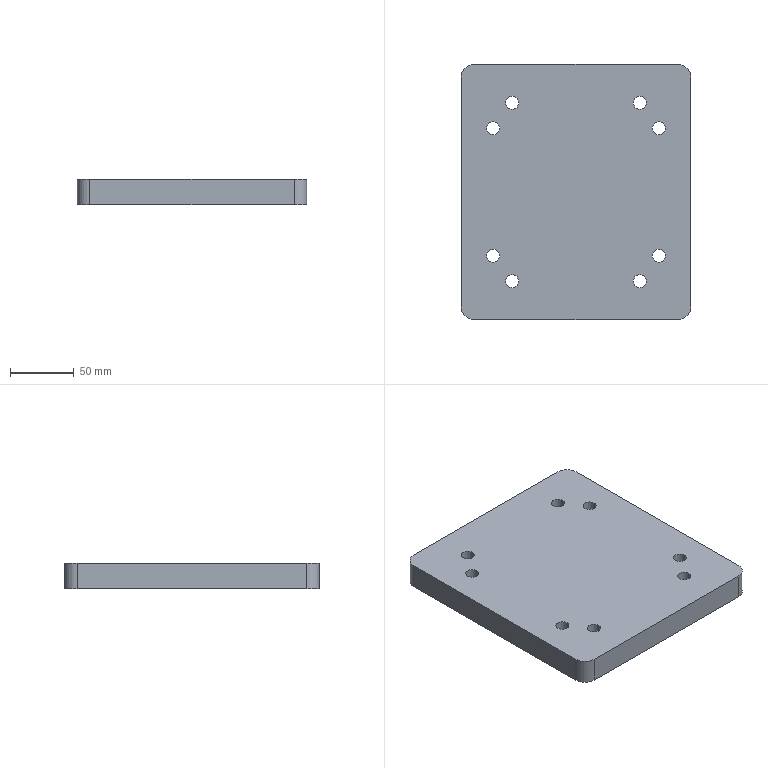Part | SolidWorks | features BaseBody 1 | 1 solid | 26 faces | box 180 x 200 x 20 mm | volume 705209 mm3 | cylinder 20 | plane 6 | commonest cylinder face diameters 10.2 x16 20 x4
STEP:
#1=CARTESIAN_POINT('',(-55.1,70.,-10.));
#2=VERTEX_POINT('',#1);
#3=CARTESIAN_POINT('',(-44.9,70.,-10.));
#4=VERTEX_POINT('',#3);
#5=CARTESIAN_POINT('',(-50.,70.,-10.));
#6=DIRECTION('',(0.,0.,1.));
#7=DIRECTION('',(1.,0.,0.));
#8=AXIS2_PLACEMENT_3D('',#5,#6,#7);
#9=CIRCLE('',#8,5.1);
#10=EDGE_CURVE('',#2,#4,#9,.T.);
#11=ORIENTED_EDGE('',*,*,#10,.F.);
#12=CARTESIAN_POINT('',(-55.1,70.,10.));
#13=VERTEX_POINT('',#12);
#14=CARTESIAN_POINT('',(-55.1,70.,10.));
#15=DIRECTION('',(0.,0.,1.));
#16=VECTOR('',#15,1000.);
#17=LINE('',#14,#16);
#18=EDGE_CURVE('',#2,#13,#17,.T.);
#19=ORIENTED_EDGE('',*,*,#18,.T.);
#20=CARTESIAN_POINT('',(-44.9,70.,10.));
#21=VERTEX_POINT('',#20);
#22=CARTESIAN_POINT('',(-50.,70.,10.));
#23=DIRECTION('',(0.,0.,1.));
#24=DIRECTION('',(1.,0.,0.));
#25=AXIS2_PLACEMENT_3D('',#22,#23,#24);
#26=CIRCLE('',#25,5.1);
#27=EDGE_CURVE('',#13,#21,#26,.T.);
#28=ORIENTED_EDGE('',*,*,#27,.T.);
#29=CARTESIAN_POINT('',(-44.9,70.,10.));
#30=DIRECTION('',(0.,0.,1.));
#31=VECTOR('',#30,1000.);
#32=LINE('',#29,#31);
#33=EDGE_CURVE('',#4,#21,#32,.T.);
#34=ORIENTED_EDGE('',*,*,#33,.F.);
#35=EDGE_LOOP('',(#11,#19,#28,#34));
#36=FACE_OUTER_BOUND('',#35,.T.);
#37=CARTESIAN_POINT('',(-50.,70.,10.));
#38=DIRECTION('',(0.,0.,1.));
#39=DIRECTION('',(1.,0.,0.));
#40=AXIS2_PLACEMENT_3D('',#37,#38,#39);
#41=CYLINDRICAL_SURFACE('',#40,5.1);
#42=ADVANCED_FACE('',(#36),#41,.F.);
#43=CARTESIAN_POINT('',(44.9,70.,-10.));
#44=VERTEX_POINT('',#43);
#45=CARTESIAN_POINT('',(55.1,70.,-10.));
#46=VERTEX_POINT('',#45);
#47=CARTESIAN_POINT('',(50.,70.,-10.));
#48=DIRECTION('',(0.,0.,1.));
#49=DIRECTION('',(1.,0.,0.));
#50=AXIS2_PLACEMENT_3D('',#47,#48,#49);
#51=CIRCLE('',#50,5.1);
#52=EDGE_CURVE('',#44,#46,#51,.T.);
#53=ORIENTED_EDGE('',*,*,#52,.F.);
#54=CARTESIAN_POINT('',(44.9,70.,10.));
#55=VERTEX_POINT('',#54);
#56=CARTESIAN_POINT('',(44.9,70.,10.));
#57=DIRECTION('',(0.,0.,1.));
#58=VECTOR('',#57,1000.);
#59=LINE('',#56,#58);
#60=EDGE_CURVE('',#44,#55,#59,.T.);
#61=ORIENTED_EDGE('',*,*,#60,.T.);
#62=CARTESIAN_POINT('',(55.1,70.,10.));
#63=VERTEX_POINT('',#62);
#64=CARTESIAN_POINT('',(50.,70.,10.));
#65=DIRECTION('',(0.,0.,1.));
#66=DIRECTION('',(1.,0.,0.));
#67=AXIS2_PLACEMENT_3D('',#64,#65,#66);
#68=CIRCLE('',#67,5.1);
#69=EDGE_CURVE('',#55,#63,#68,.T.);
#70=ORIENTED_EDGE('',*,*,#69,.T.);
#71=CARTESIAN_POINT('',(55.1,70.,10.));
#72=DIRECTION('',(0.,0.,1.));
#73=VECTOR('',#72,1000.);
#74=LINE('',#71,#73);
#75=EDGE_CURVE('',#46,#63,#74,.T.);
#76=ORIENTED_EDGE('',*,*,#75,.F.);
#77=EDGE_LOOP('',(#53,#61,#70,#76));
#78=FACE_OUTER_BOUND('',#77,.T.);
#79=CARTESIAN_POINT('',(50.,70.,10.));
#80=DIRECTION('',(0.,0.,1.));
#81=DIRECTION('',(1.,0.,0.));
#82=AXIS2_PLACEMENT_3D('',#79,#80,#81);
#83=CYLINDRICAL_SURFACE('',#82,5.1);
#84=ADVANCED_FACE('',(#78),#83,.F.);
#85=CARTESIAN_POINT('',(44.9,-70.,-10.));
#86=VERTEX_POINT('',#85);
#87=CARTESIAN_POINT('',(55.1,-70.,-10.));
#88=VERTEX_POINT('',#87);
#89=CARTESIAN_POINT('',(50.,-70.,-10.));
#90=DIRECTION('',(0.,0.,1.));
#91=DIRECTION('',(1.,0.,0.));
#92=AXIS2_PLACEMENT_3D('',#89,#90,#91);
#93=CIRCLE('',#92,5.1);
#94=EDGE_CURVE('',#86,#88,#93,.T.);
#95=ORIENTED_EDGE('',*,*,#94,.F.);
#96=CARTESIAN_POINT('',(44.9,-70.,10.));
#97=VERTEX_POINT('',#96);
#98=CARTESIAN_POINT('',(44.9,-70.,10.));
#99=DIRECTION('',(0.,0.,1.));
#100=VECTOR('',#99,1000.);
#101=LINE('',#98,#100);
#102=EDGE_CURVE('',#86,#97,#101,.T.);
#103=ORIENTED_EDGE('',*,*,#102,.T.);
#104=CARTESIAN_POINT('',(55.1,-70.,10.));
#105=VERTEX_POINT('',#104);
#106=CARTESIAN_POINT('',(50.,-70.,10.));
#107=DIRECTION('',(0.,0.,1.));
#108=DIRECTION('',(1.,0.,0.));
#109=AXIS2_PLACEMENT_3D('',#106,#107,#108);
#110=CIRCLE('',#109,5.1);
#111=EDGE_CURVE('',#97,#105,#110,.T.);
#112=ORIENTED_EDGE('',*,*,#111,.T.);
#113=CARTESIAN_POINT('',(55.1,-70.,10.));
#114=DIRECTION('',(0.,0.,1.));
#115=VECTOR('',#114,1000.);
#116=LINE('',#113,#115);
#117=EDGE_CURVE('',#88,#105,#116,.T.);
#118=ORIENTED_EDGE('',*,*,#117,.F.);
#119=EDGE_LOOP('',(#95,#103,#112,#118));
#120=FACE_OUTER_BOUND('',#119,.T.);
#121=CARTESIAN_POINT('',(50.,-70.,10.));
#122=DIRECTION('',(0.,0.,1.));
#123=DIRECTION('',(1.,0.,0.));
#124=AXIS2_PLACEMENT_3D('',#121,#122,#123);
#125=CYLINDRICAL_SURFACE('',#124,5.1);
#126=ADVANCED_FACE('',(#120),#125,.F.);
#127=CARTESIAN_POINT('',(-55.1,-70.,-10.));
#128=VERTEX_POINT('',#127);
#129=CARTESIAN_POINT('',(-44.9,-70.,-10.));
#130=VERTEX_POINT('',#129);
#131=CARTESIAN_POINT('',(-50.,-70.,-10.));
#132=DIRECTION('',(0.,0.,1.));
#133=DIRECTION('',(1.,0.,0.));
#134=AXIS2_PLACEMENT_3D('',#131,#132,#133);
#135=CIRCLE('',#134,5.1);
#136=EDGE_CURVE('',#128,#130,#135,.T.);
#137=ORIENTED_EDGE('',*,*,#136,.F.);
#138=CARTESIAN_POINT('',(-55.1,-70.,10.));
#139=VERTEX_POINT('',#138);
#140=CARTESIAN_POINT('',(-55.1,-70.,10.));
#141=DIRECTION('',(0.,0.,1.));
#142=VECTOR('',#141,1000.);
#143=LINE('',#140,#142);
#144=EDGE_CURVE('',#128,#139,#143,.T.);
#145=ORIENTED_EDGE('',*,*,#144,.T.);
#146=CARTESIAN_POINT('',(-44.9,-70.,10.));
#147=VERTEX_POINT('',#146);
#148=CARTESIAN_POINT('',(-50.,-70.,10.));
#149=DIRECTION('',(0.,0.,1.));
#150=DIRECTION('',(1.,0.,0.));
#151=AXIS2_PLACEMENT_3D('',#148,#149,#150);
#152=CIRCLE('',#151,5.1);
#153=EDGE_CURVE('',#139,#147,#152,.T.);
#154=ORIENTED_EDGE('',*,*,#153,.T.);
#155=CARTESIAN_POINT('',(-44.9,-70.,10.));
#156=DIRECTION('',(0.,0.,1.));
#157=VECTOR('',#156,1000.);
#158=LINE('',#155,#157);
#159=EDGE_CURVE('',#130,#147,#158,.T.);
#160=ORIENTED_EDGE('',*,*,#159,.F.);
#161=EDGE_LOOP('',(#137,#145,#154,#160));
#162=FACE_OUTER_BOUND('',#161,.T.);
#163=CARTESIAN_POINT('',(-50.,-70.,10.));
#164=DIRECTION('',(0.,0.,1.));
#165=DIRECTION('',(1.,0.,0.));
#166=AXIS2_PLACEMENT_3D('',#163,#164,#165);
#167=CYLINDRICAL_SURFACE('',#166,5.1);
#168=ADVANCED_FACE('',(#162),#167,.F.);
#169=CARTESIAN_POINT('',(-70.1,50.,-10.));
#170=VERTEX_POINT('',#169);
#171=CARTESIAN_POINT('',(-59.9,50.,-10.));
#172=VERTEX_POINT('',#171);
#173=CARTESIAN_POINT('',(-65.,50.,-10.));
#174=DIRECTION('',(0.,0.,1.));
#175=DIRECTION('',(1.,0.,0.));
#176=AXIS2_PLACEMENT_3D('',#173,#174,#175);
#177=CIRCLE('',#176,5.1);
#178=EDGE_CURVE('',#170,#172,#177,.T.);
#179=ORIENTED_EDGE('',*,*,#178,.F.);
#180=CARTESIAN_POINT('',(-70.1,50.,10.));
#181=VERTEX_POINT('',#180);
#182=CARTESIAN_POINT('',(-70.1,50.,10.));
#183=DIRECTION('',(0.,0.,1.));
#184=VECTOR('',#183,1000.);
#185=LINE('',#182,#184);
#186=EDGE_CURVE('',#170,#181,#185,.T.);
#187=ORIENTED_EDGE('',*,*,#186,.T.);
#188=CARTESIAN_POINT('',(-59.9,50.,10.));
#189=VERTEX_POINT('',#188);
#190=CARTESIAN_POINT('',(-65.,50.,10.));
#191=DIRECTION('',(0.,0.,1.));
#192=DIRECTION('',(1.,0.,0.));
#193=AXIS2_PLACEMENT_3D('',#190,#191,#192);
#194=CIRCLE('',#193,5.1);
#195=EDGE_CURVE('',#181,#189,#194,.T.);
#196=ORIENTED_EDGE('',*,*,#195,.T.);
#197=CARTESIAN_POINT('',(-59.9,50.,10.));
#198=DIRECTION('',(0.,0.,1.));
#199=VECTOR('',#198,1000.);
#200=LINE('',#197,#199);
#201=EDGE_CURVE('',#172,#189,#200,.T.);
#202=ORIENTED_EDGE('',*,*,#201,.F.);
#203=EDGE_LOOP('',(#179,#187,#196,#202));
#204=FACE_OUTER_BOUND('',#203,.T.);
#205=CARTESIAN_POINT('',(-65.,50.,10.));
#206=DIRECTION('',(0.,0.,1.));
#207=DIRECTION('',(1.,0.,0.));
#208=AXIS2_PLACEMENT_3D('',#205,#206,#207);
#209=CYLINDRICAL_SURFACE('',#208,5.1);
#210=ADVANCED_FACE('',(#204),#209,.F.);
#211=CARTESIAN_POINT('',(59.9,50.,-10.));
#212=VERTEX_POINT('',#211);
#213=CARTESIAN_POINT('',(70.1,50.,-10.));
#214=VERTEX_POINT('',#213);
#215=CARTESIAN_POINT('',(65.,50.,-10.));
#216=DIRECTION('',(0.,0.,1.));
#217=DIRECTION('',(1.,0.,0.));
#218=AXIS2_PLACEMENT_3D('',#215,#216,#217);
#219=CIRCLE('',#218,5.1);
#220=EDGE_CURVE('',#212,#214,#219,.T.);
#221=ORIENTED_EDGE('',*,*,#220,.F.);
#222=CARTESIAN_POINT('',(59.9,50.,10.));
#223=VERTEX_POINT('',#222);
#224=CARTESIAN_POINT('',(59.9,50.,10.));
#225=DIRECTION('',(0.,0.,1.));
#226=VECTOR('',#225,1000.);
#227=LINE('',#224,#226);
#228=EDGE_CURVE('',#212,#223,#227,.T.);
#229=ORIENTED_EDGE('',*,*,#228,.T.);
#230=CARTESIAN_POINT('',(70.1,50.,10.));
#231=VERTEX_POINT('',#230);
#232=CARTESIAN_POINT('',(65.,50.,10.));
#233=DIRECTION('',(0.,0.,1.));
#234=DIRECTION('',(1.,0.,0.));
#235=AXIS2_PLACEMENT_3D('',#232,#233,#234);
#236=CIRCLE('',#235,5.1);
#237=EDGE_CURVE('',#223,#231,#236,.T.);
#238=ORIENTED_EDGE('',*,*,#237,.T.);
#239=CARTESIAN_POINT('',(70.1,50.,10.));
#240=DIRECTION('',(0.,0.,1.));
#241=VECTOR('',#240,1000.);
#242=LINE('',#239,#241);
#243=EDGE_CURVE('',#214,#231,#242,.T.);
#244=ORIENTED_EDGE('',*,*,#243,.F.);
#245=EDGE_LOOP('',(#221,#229,#238,#244));
#246=FACE_OUTER_BOUND('',#245,.T.);
#247=CARTESIAN_POINT('',(65.,50.,10.));
#248=DIRECTION('',(0.,0.,1.));
#249=DIRECTION('',(1.,0.,0.));
#250=AXIS2_PLACEMENT_3D('',#247,#248,#249);
#251=CYLINDRICAL_SURFACE('',#250,5.1);
#252=ADVANCED_FACE('',(#246),#251,.F.);
#253=CARTESIAN_POINT('',(59.9,-50.,-10.));
#254=VERTEX_POINT('',#253);
#255=CARTESIAN_POINT('',(70.1,-50.,-10.));
#256=VERTEX_POINT('',#255);
#257=CARTESIAN_POINT('',(65.,-50.,-10.));
#258=DIRECTION('',(0.,0.,1.));
#259=DIRECTION('',(1.,0.,0.));
#260=AXIS2_PLACEMENT_3D('',#257,#258,#259);
#261=CIRCLE('',#260,5.1);
#262=EDGE_CURVE('',#254,#256,#261,.T.);
#263=ORIENTED_EDGE('',*,*,#262,.F.);
#264=CARTESIAN_POINT('',(59.9,-50.,10.));
#265=VERTEX_POINT('',#264);
#266=CARTESIAN_POINT('',(59.9,-50.,10.));
#267=DIRECTION('',(0.,0.,1.));
#268=VECTOR('',#267,1000.);
#269=LINE('',#266,#268);
#270=EDGE_CURVE('',#254,#265,#269,.T.);
#271=ORIENTED_EDGE('',*,*,#270,.T.);
#272=CARTESIAN_POINT('',(70.1,-50.,10.));
#273=VERTEX_POINT('',#272);
#274=CARTESIAN_POINT('',(65.,-50.,10.));
#275=DIRECTION('',(0.,0.,1.));
#276=DIRECTION('',(1.,0.,0.));
#277=AXIS2_PLACEMENT_3D('',#274,#275,#276);
#278=CIRCLE('',#277,5.1);
#279=EDGE_CURVE('',#265,#273,#278,.T.);
#280=ORIENTED_EDGE('',*,*,#279,.T.);
#281=CARTESIAN_POINT('',(70.1,-50.,10.));
#282=DIRECTION('',(0.,0.,1.));
#283=VECTOR('',#282,1000.);
#284=LINE('',#281,#283);
#285=EDGE_CURVE('',#256,#273,#284,.T.);
#286=ORIENTED_EDGE('',*,*,#285,.F.);
#287=EDGE_LOOP('',(#263,#271,#280,#286));
#288=FACE_OUTER_BOUND('',#287,.T.);
#289=CARTESIAN_POINT('',(65.,-50.,10.));
#290=DIRECTION('',(0.,0.,1.));
#291=DIRECTION('',(1.,0.,0.));
#292=AXIS2_PLACEMENT_3D('',#289,#290,#291);
#293=CYLINDRICAL_SURFACE('',#292,5.1);
#294=ADVANCED_FACE('',(#288),#293,.F.);
#295=CARTESIAN_POINT('',(-70.1,-50.,-10.));
#296=VERTEX_POINT('',#295);
#297=CARTESIAN_POINT('',(-59.9,-50.,-10.));
#298=VERTEX_POINT('',#297);
#299=CARTESIAN_POINT('',(-65.,-50.,-10.));
#300=DIRECTION('',(0.,0.,1.));
#301=DIRECTION('',(1.,0.,0.));
#302=AXIS2_PLACEMENT_3D('',#299,#300,#301);
#303=CIRCLE('',#302,5.1);
#304=EDGE_CURVE('',#296,#298,#303,.T.);
#305=ORIENTED_EDGE('',*,*,#304,.F.);
#306=CARTESIAN_POINT('',(-70.1,-50.,10.));
#307=VERTEX_POINT('',#306);
#308=CARTESIAN_POINT('',(-70.1,-50.,10.));
#309=DIRECTION('',(0.,0.,1.));
#310=VECTOR('',#309,1000.);
#311=LINE('',#308,#310);
#312=EDGE_CURVE('',#296,#307,#311,.T.);
#313=ORIENTED_EDGE('',*,*,#312,.T.);
#314=CARTESIAN_POINT('',(-59.9,-50.,10.));
#315=VERTEX_POINT('',#314);
#316=CARTESIAN_POINT('',(-65.,-50.,10.));
#317=DIRECTION('',(0.,0.,1.));
#318=DIRECTION('',(1.,0.,0.));
#319=AXIS2_PLACEMENT_3D('',#316,#317,#318);
#320=CIRCLE('',#319,5.1);
#321=EDGE_CURVE('',#307,#315,#320,.T.);
#322=ORIENTED_EDGE('',*,*,#321,.T.);
#323=CARTESIAN_POINT('',(-59.9,-50.,10.));
#324=DIRECTION('',(0.,0.,1.));
#325=VECTOR('',#324,1000.);
#326=LINE('',#323,#325);
#327=EDGE_CURVE('',#298,#315,#326,.T.);
#328=ORIENTED_EDGE('',*,*,#327,.F.);
#329=EDGE_LOOP('',(#305,#313,#322,#328));
#330=FACE_OUTER_BOUND('',#329,.T.);
#331=CARTESIAN_POINT('',(-65.,-50.,10.));
#332=DIRECTION('',(0.,0.,1.));
#333=DIRECTION('',(1.,0.,0.));
#334=AXIS2_PLACEMENT_3D('',#331,#332,#333);
#335=CYLINDRICAL_SURFACE('',#334,5.1);
#336=ADVANCED_FACE('',(#330),#335,.F.);
#337=CARTESIAN_POINT('',(90.,90.,-10.));
#338=VERTEX_POINT('',#337);
#339=CARTESIAN_POINT('',(80.,100.,-10.));
#340=VERTEX_POINT('',#339);
#341=CARTESIAN_POINT('',(80.,90.,-10.));
#342=DIRECTION('',(0.,0.,1.));
#343=DIRECTION('',(-1.,0.,0.));
#344=AXIS2_PLACEMENT_3D('',#341,#342,#343);
#345=CIRCLE('',#344,10.);
#346=EDGE_CURVE('',#338,#340,#345,.T.);
#347=ORIENTED_EDGE('',*,*,#346,.T.);
#348=CARTESIAN_POINT('',(80.,100.,10.));
#349=VERTEX_POINT('',#348);
#350=CARTESIAN_POINT('',(80.,100.,10.));
#351=DIRECTION('',(0.,0.,-1.));
#352=VECTOR('',#351,1000.);
#353=LINE('',#350,#352);
#354=EDGE_CURVE('',#349,#340,#353,.T.);
#355=ORIENTED_EDGE('',*,*,#354,.F.);
#356=CARTESIAN_POINT('',(90.,90.,10.));
#357=VERTEX_POINT('',#356);
#358=CARTESIAN_POINT('',(80.,90.,10.));
#359=DIRECTION('',(0.,0.,1.));
#360=DIRECTION('',(-1.,0.,0.));
#361=AXIS2_PLACEMENT_3D('',#358,#359,#360);
#362=CIRCLE('',#361,10.);
#363=EDGE_CURVE('',#357,#349,#362,.T.);
#364=ORIENTED_EDGE('',*,*,#363,.F.);
#365=CARTESIAN_POINT('',(90.,90.,10.));
#366=DIRECTION('',(0.,0.,-1.));
#367=VECTOR('',#366,1000.);
#368=LINE('',#365,#367);
#369=EDGE_CURVE('',#357,#338,#368,.T.);
#370=ORIENTED_EDGE('',*,*,#369,.T.);
#371=EDGE_LOOP('',(#347,#355,#364,#370));
#372=FACE_OUTER_BOUND('',#371,.T.);
#373=CARTESIAN_POINT('',(80.,90.,10.));
#374=DIRECTION('',(0.,0.,-1.));
#375=DIRECTION('',(-1.,0.,0.));
#376=AXIS2_PLACEMENT_3D('',#373,#374,#375);
#377=CYLINDRICAL_SURFACE('',#376,10.);
#378=ADVANCED_FACE('',(#372),#377,.T.);
#379=CARTESIAN_POINT('',(-80.,100.,-10.));
#380=VERTEX_POINT('',#379);
#381=CARTESIAN_POINT('',(-80.,100.,-10.));
#382=DIRECTION('',(-1.,0.,0.));
#383=VECTOR('',#382,1000.);
#384=LINE('',#381,#383);
#385=EDGE_CURVE('',#340,#380,#384,.T.);
#386=ORIENTED_EDGE('',*,*,#385,.T.);
#387=CARTESIAN_POINT('',(-80.,100.,10.));
#388=VERTEX_POINT('',#387);
#389=CARTESIAN_POINT('',(-80.,100.,10.));
#390=DIRECTION('',(0.,0.,-1.));
#391=VECTOR('',#390,1000.);
#392=LINE('',#389,#391);
#393=EDGE_CURVE('',#388,#380,#392,.T.);
#394=ORIENTED_EDGE('',*,*,#393,.F.);
#395=CARTESIAN_POINT('',(-80.,100.,10.));
#396=DIRECTION('',(-1.,0.,0.));
#397=VECTOR('',#396,1000.);
#398=LINE('',#395,#397);
#399=EDGE_CURVE('',#349,#388,#398,.T.);
#400=ORIENTED_EDGE('',*,*,#399,.F.);
#401=ORIENTED_EDGE('',*,*,#354,.T.);
#402=EDGE_LOOP('',(#386,#394,#400,#401));
#403=FACE_OUTER_BOUND('',#402,.T.);
#404=CARTESIAN_POINT('',(-80.,100.,10.));
#405=DIRECTION('',(0.,-1.,0.));
#406=DIRECTION('',(0.,0.,-1.));
#407=AXIS2_PLACEMENT_3D('',#404,#405,#406);
#408=PLANE('',#407);
#409=ADVANCED_FACE('',(#403),#408,.F.);
#410=CARTESIAN_POINT('',(-90.,90.,-10.));
#411=VERTEX_POINT('',#410);
#412=CARTESIAN_POINT('',(-80.,90.,-10.));
#413=DIRECTION('',(0.,0.,1.));
#414=DIRECTION('',(1.,0.,0.));
#415=AXIS2_PLACEMENT_3D('',#412,#413,#414);
#416=CIRCLE('',#415,10.);
#417=EDGE_CURVE('',#380,#411,#416,.T.);
#418=ORIENTED_EDGE('',*,*,#417,.T.);
#419=CARTESIAN_POINT('',(-90.,90.,10.));
#420=VERTEX_POINT('',#419);
#421=CARTESIAN_POINT('',(-90.,90.,10.));
#422=DIRECTION('',(0.,0.,-1.));
#423=VECTOR('',#422,1000.);
#424=LINE('',#421,#423);
#425=EDGE_CURVE('',#420,#411,#424,.T.);
#426=ORIENTED_EDGE('',*,*,#425,.F.);
#427=CARTESIAN_POINT('',(-80.,90.,10.));
#428=DIRECTION('',(0.,0.,1.));
#429=DIRECTION('',(1.,0.,0.));
#430=AXIS2_PLACEMENT_3D('',#427,#428,#429);
#431=CIRCLE('',#430,10.);
#432=EDGE_CURVE('',#388,#420,#431,.T.);
#433=ORIENTED_EDGE('',*,*,#432,.F.);
#434=ORIENTED_EDGE('',*,*,#393,.T.);
#435=EDGE_LOOP('',(#418,#426,#433,#434));
#436=FACE_OUTER_BOUND('',#435,.T.);
#437=CARTESIAN_POINT('',(-80.,90.,10.));
#438=DIRECTION('',(0.,0.,-1.));
#439=DIRECTION('',(-1.,0.,0.));
#440=AXIS2_PLACEMENT_3D('',#437,#438,#439);
#441=CYLINDRICAL_SURFACE('',#440,10.);
#442=ADVANCED_FACE('',(#436),#441,.T.);
#443=CARTESIAN_POINT('',(-90.,-90.,-10.));
#444=VERTEX_POINT('',#443);
#445=CARTESIAN_POINT('',(-90.,90.,-10.));
#446=DIRECTION('',(0.,-1.,0.));
#447=VECTOR('',#446,1000.);
#448=LINE('',#445,#447);
#449=EDGE_CURVE('',#411,#444,#448,.T.);
#450=ORIENTED_EDGE('',*,*,#449,.T.);
#451=CARTESIAN_POINT('',(-90.,-90.,10.));
#452=VERTEX_POINT('',#451);
#453=CARTESIAN_POINT('',(-90.,-90.,10.));
#454=DIRECTION('',(0.,0.,-1.));
#455=VECTOR('',#454,1000.);
#456=LINE('',#453,#455);
#457=EDGE_CURVE('',#452,#444,#456,.T.);
#458=ORIENTED_EDGE('',*,*,#457,.F.);
#459=CARTESIAN_POINT('',(-90.,90.,10.));
#460=DIRECTION('',(0.,-1.,0.));
#461=VECTOR('',#460,1000.);
#462=LINE('',#459,#461);
#463=EDGE_CURVE('',#420,#452,#462,.T.);
#464=ORIENTED_EDGE('',*,*,#463,.F.);
#465=ORIENTED_EDGE('',*,*,#425,.T.);
#466=EDGE_LOOP('',(#450,#458,#464,#465));
#467=FACE_OUTER_BOUND('',#466,.T.);
#468=CARTESIAN_POINT('',(-90.,90.,10.));
#469=DIRECTION('',(1.,0.,0.));
#470=DIRECTION('',(0.,1.,0.));
#471=AXIS2_PLACEMENT_3D('',#468,#469,#470);
#472=PLANE('',#471);
#473=ADVANCED_FACE('',(#467),#472,.F.);
#474=CARTESIAN_POINT('',(-80.,-100.,-10.));
#475=VERTEX_POINT('',#474);
#476=CARTESIAN_POINT('',(-80.,-90.,-10.));
#477=DIRECTION('',(0.,0.,1.));
#478=DIRECTION('',(1.,0.,0.));
#479=AXIS2_PLACEMENT_3D('',#476,#477,#478);
#480=CIRCLE('',#479,10.);
#481=EDGE_CURVE('',#444,#475,#480,.T.);
#482=ORIENTED_EDGE('',*,*,#481,.T.);
#483=CARTESIAN_POINT('',(-80.,-100.,10.));
#484=VERTEX_POINT('',#483);
#485=CARTESIAN_POINT('',(-80.,-100.,10.));
#486=DIRECTION('',(0.,0.,-1.));
#487=VECTOR('',#486,1000.);
#488=LINE('',#485,#487);
#489=EDGE_CURVE('',#484,#475,#488,.T.);
#490=ORIENTED_EDGE('',*,*,#489,.F.);
#491=CARTESIAN_POINT('',(-80.,-90.,10.));
#492=DIRECTION('',(0.,0.,1.));
#493=DIRECTION('',(1.,0.,0.));
#494=AXIS2_PLACEMENT_3D('',#491,#492,#493);
#495=CIRCLE('',#494,10.);
#496=EDGE_CURVE('',#452,#484,#495,.T.);
#497=ORIENTED_EDGE('',*,*,#496,.F.);
#498=ORIENTED_EDGE('',*,*,#457,.T.);
#499=EDGE_LOOP('',(#482,#490,#497,#498));
#500=FACE_OUTER_BOUND('',#499,.T.);
#501=CARTESIAN_POINT('',(-80.,-90.,10.));
#502=DIRECTION('',(0.,0.,-1.));
#503=DIRECTION('',(-1.,0.,0.));
#504=AXIS2_PLACEMENT_3D('',#501,#502,#503);
#505=CYLINDRICAL_SURFACE('',#504,10.);
#506=ADVANCED_FACE('',(#500),#505,.T.);
#507=CARTESIAN_POINT('',(80.,-100.,-10.));
#508=VERTEX_POINT('',#507);
#509=CARTESIAN_POINT('',(-80.,-100.,-10.));
#510=DIRECTION('',(1.,0.,0.));
#511=VECTOR('',#510,1000.);
#512=LINE('',#509,#511);
#513=EDGE_CURVE('',#475,#508,#512,.T.);
#514=ORIENTED_EDGE('',*,*,#513,.T.);
#515=CARTESIAN_POINT('',(80.,-100.,10.));
#516=VERTEX_POINT('',#515);
#517=CARTESIAN_POINT('',(80.,-100.,10.));
#518=DIRECTION('',(0.,0.,-1.));
#519=VECTOR('',#518,1000.);
#520=LINE('',#517,#519);
#521=EDGE_CURVE('',#516,#508,#520,.T.);
#522=ORIENTED_EDGE('',*,*,#521,.F.);
#523=CARTESIAN_POINT('',(-80.,-100.,10.));
#524=DIRECTION('',(1.,0.,0.));
#525=VECTOR('',#524,1000.);
#526=LINE('',#523,#525);
#527=EDGE_CURVE('',#484,#516,#526,.T.);
#528=ORIENTED_EDGE('',*,*,#527,.F.);
#529=ORIENTED_EDGE('',*,*,#489,.T.);
#530=EDGE_LOOP('',(#514,#522,#528,#529));
#531=FACE_OUTER_BOUND('',#530,.T.);
#532=CARTESIAN_POINT('',(-80.,-100.,10.));
#533=DIRECTION('',(0.,1.,0.));
#534=DIRECTION('',(0.,0.,1.));
#535=AXIS2_PLACEMENT_3D('',#532,#533,#534);
#536=PLANE('',#535);
#537=ADVANCED_FACE('',(#531),#536,.F.);
#538=CARTESIAN_POINT('',(90.,-90.,-10.));
#539=VERTEX_POINT('',#538);
#540=CARTESIAN_POINT('',(80.,-90.,-10.));
#541=DIRECTION('',(0.,0.,1.));
#542=DIRECTION('',(1.,0.,0.));
#543=AXIS2_PLACEMENT_3D('',#540,#541,#542);
#544=CIRCLE('',#543,10.);
#545=EDGE_CURVE('',#508,#539,#544,.T.);
#546=ORIENTED_EDGE('',*,*,#545,.T.);
#547=CARTESIAN_POINT('',(90.,-90.,10.));
#548=VERTEX_POINT('',#547);
#549=CARTESIAN_POINT('',(90.,-90.,10.));
#550=DIRECTION('',(0.,0.,-1.));
#551=VECTOR('',#550,1000.);
#552=LINE('',#549,#551);
#553=EDGE_CURVE('',#548,#539,#552,.T.);
#554=ORIENTED_EDGE('',*,*,#553,.F.);
#555=CARTESIAN_POINT('',(80.,-90.,10.));
#556=DIRECTION('',(0.,0.,1.));
#557=DIRECTION('',(1.,0.,0.));
#558=AXIS2_PLACEMENT_3D('',#555,#556,#557);
#559=CIRCLE('',#558,10.);
#560=EDGE_CURVE('',#516,#548,#559,.T.);
#561=ORIENTED_EDGE('',*,*,#560,.F.);
#562=ORIENTED_EDGE('',*,*,#521,.T.);
#563=EDGE_LOOP('',(#546,#554,#561,#562));
#564=FACE_OUTER_BOUND('',#563,.T.);
#565=CARTESIAN_POINT('',(80.,-90.,10.));
#566=DIRECTION('',(0.,0.,-1.));
#567=DIRECTION('',(-1.,0.,0.));
#568=AXIS2_PLACEMENT_3D('',#565,#566,#567);
#569=CYLINDRICAL_SURFACE('',#568,10.);
#570=ADVANCED_FACE('',(#564),#569,.T.);
#571=CARTESIAN_POINT('',(90.,90.,-10.));
#572=DIRECTION('',(0.,1.,0.));
#573=VECTOR('',#572,1000.);
#574=LINE('',#571,#573);
#575=EDGE_CURVE('',#539,#338,#574,.T.);
#576=ORIENTED_EDGE('',*,*,#575,.T.);
#577=ORIENTED_EDGE('',*,*,#369,.F.);
#578=CARTESIAN_POINT('',(90.,90.,10.));
#579=DIRECTION('',(0.,1.,0.));
#580=VECTOR('',#579,1000.);
#581=LINE('',#578,#580);
#582=EDGE_CURVE('',#548,#357,#581,.T.);
#583=ORIENTED_EDGE('',*,*,#582,.F.);
#584=ORIENTED_EDGE('',*,*,#553,.T.);
#585=EDGE_LOOP('',(#576,#577,#583,#584));
#586=FACE_OUTER_BOUND('',#585,.T.);
#587=CARTESIAN_POINT('',(90.,90.,10.));
#588=DIRECTION('',(-1.,0.,0.));
#589=DIRECTION('',(0.,-1.,0.));
#590=AXIS2_PLACEMENT_3D('',#587,#588,#589);
#591=PLANE('',#590);
#592=ADVANCED_FACE('',(#586),#591,.F.);
#593=CARTESIAN_POINT('',(-50.,70.,10.));
#594=DIRECTION('',(0.,0.,1.));
#595=DIRECTION('',(1.,0.,0.));
#596=AXIS2_PLACEMENT_3D('',#593,#594,#595);
#597=CIRCLE('',#596,5.1);
#598=EDGE_CURVE('',#21,#13,#597,.T.);
#599=ORIENTED_EDGE('',*,*,#598,.F.);
#600=ORIENTED_EDGE('',*,*,#27,.F.);
#601=EDGE_LOOP('',(#599,#600));
#602=FACE_BOUND('',#601,.T.);
#603=CARTESIAN_POINT('',(50.,70.,10.));
#604=DIRECTION('',(0.,0.,1.));
#605=DIRECTION('',(1.,0.,0.));
#606=AXIS2_PLACEMENT_3D('',#603,#604,#605);
#607=CIRCLE('',#606,5.1);
#608=EDGE_CURVE('',#63,#55,#607,.T.);
#609=ORIENTED_EDGE('',*,*,#608,.F.);
#610=ORIENTED_EDGE('',*,*,#69,.F.);
#611=EDGE_LOOP('',(#609,#610));
#612=FACE_BOUND('',#611,.T.);
#613=CARTESIAN_POINT('',(50.,-70.,10.));
#614=DIRECTION('',(0.,0.,1.));
#615=DIRECTION('',(1.,0.,0.));
#616=AXIS2_PLACEMENT_3D('',#613,#614,#615);
#617=CIRCLE('',#616,5.1);
#618=EDGE_CURVE('',#105,#97,#617,.T.);
#619=ORIENTED_EDGE('',*,*,#618,.F.);
#620=ORIENTED_EDGE('',*,*,#111,.F.);
#621=EDGE_LOOP('',(#619,#620));
#622=FACE_BOUND('',#621,.T.);
#623=CARTESIAN_POINT('',(-50.,-70.,10.));
#624=DIRECTION('',(0.,0.,1.));
#625=DIRECTION('',(1.,0.,0.));
#626=AXIS2_PLACEMENT_3D('',#623,#624,#625);
#627=CIRCLE('',#626,5.1);
#628=EDGE_CURVE('',#147,#139,#627,.T.);
#629=ORIENTED_EDGE('',*,*,#628,.F.);
#630=ORIENTED_EDGE('',*,*,#153,.F.);
#631=EDGE_LOOP('',(#629,#630));
#632=FACE_BOUND('',#631,.T.);
#633=CARTESIAN_POINT('',(-65.,50.,10.));
#634=DIRECTION('',(0.,0.,1.));
#635=DIRECTION('',(1.,0.,0.));
#636=AXIS2_PLACEMENT_3D('',#633,#634,#635);
#637=CIRCLE('',#636,5.1);
#638=EDGE_CURVE('',#189,#181,#637,.T.);
#639=ORIENTED_EDGE('',*,*,#638,.F.);
#640=ORIENTED_EDGE('',*,*,#195,.F.);
#641=EDGE_LOOP('',(#639,#640));
#642=FACE_BOUND('',#641,.T.);
#643=CARTESIAN_POINT('',(65.,50.,10.));
#644=DIRECTION('',(0.,0.,1.));
#645=DIRECTION('',(1.,0.,0.));
#646=AXIS2_PLACEMENT_3D('',#643,#644,#645);
#647=CIRCLE('',#646,5.1);
#648=EDGE_CURVE('',#231,#223,#647,.T.);
#649=ORIENTED_EDGE('',*,*,#648,.F.);
#650=ORIENTED_EDGE('',*,*,#237,.F.);
#651=EDGE_LOOP('',(#649,#650));
#652=FACE_BOUND('',#651,.T.);
#653=CARTESIAN_POINT('',(65.,-50.,10.));
#654=DIRECTION('',(0.,0.,1.));
#655=DIRECTION('',(1.,0.,0.));
#656=AXIS2_PLACEMENT_3D('',#653,#654,#655);
#657=CIRCLE('',#656,5.1);
#658=EDGE_CURVE('',#273,#265,#657,.T.);
#659=ORIENTED_EDGE('',*,*,#658,.F.);
#660=ORIENTED_EDGE('',*,*,#279,.F.);
#661=EDGE_LOOP('',(#659,#660));
#662=FACE_BOUND('',#661,.T.);
#663=CARTESIAN_POINT('',(-65.,-50.,10.));
#664=DIRECTION('',(0.,0.,1.));
#665=DIRECTION('',(1.,0.,0.));
#666=AXIS2_PLACEMENT_3D('',#663,#664,#665);
#667=CIRCLE('',#666,5.1);
#668=EDGE_CURVE('',#315,#307,#667,.T.);
#669=ORIENTED_EDGE('',*,*,#668,.F.);
#670=ORIENTED_EDGE('',*,*,#321,.F.);
#671=EDGE_LOOP('',(#669,#670));
#672=FACE_BOUND('',#671,.T.);
#673=ORIENTED_EDGE('',*,*,#363,.T.);
#674=ORIENTED_EDGE('',*,*,#399,.T.);
#675=ORIENTED_EDGE('',*,*,#432,.T.);
#676=ORIENTED_EDGE('',*,*,#463,.T.);
#677=ORIENTED_EDGE('',*,*,#496,.T.);
#678=ORIENTED_EDGE('',*,*,#527,.T.);
#679=ORIENTED_EDGE('',*,*,#560,.T.);
#680=ORIENTED_EDGE('',*,*,#582,.T.);
#681=EDGE_LOOP('',(#673,#674,#675,#676,#677,#678,#679,#680));
#682=FACE_OUTER_BOUND('',#681,.T.);
#683=CARTESIAN_POINT('',(80.,90.,10.));
#684=DIRECTION('',(0.,0.,-1.));
#685=DIRECTION('',(-1.,0.,0.));
#686=AXIS2_PLACEMENT_3D('',#683,#684,#685);
#687=PLANE('',#686);
#688=ADVANCED_FACE('',(#602,#612,#622,#632,#642,#652,#662,#672,#682),#687,.F.);
#689=CARTESIAN_POINT('',(-50.,70.,-10.));
#690=DIRECTION('',(0.,0.,1.));
#691=DIRECTION('',(1.,0.,0.));
#692=AXIS2_PLACEMENT_3D('',#689,#690,#691);
#693=CIRCLE('',#692,5.1);
#694=EDGE_CURVE('',#4,#2,#693,.T.);
#695=ORIENTED_EDGE('',*,*,#694,.T.);
#696=ORIENTED_EDGE('',*,*,#10,.T.);
#697=EDGE_LOOP('',(#695,#696));
#698=FACE_BOUND('',#697,.T.);
#699=CARTESIAN_POINT('',(50.,70.,-10.));
#700=DIRECTION('',(0.,0.,1.));
#701=DIRECTION('',(1.,0.,0.));
#702=AXIS2_PLACEMENT_3D('',#699,#700,#701);
#703=CIRCLE('',#702,5.1);
#704=EDGE_CURVE('',#46,#44,#703,.T.);
#705=ORIENTED_EDGE('',*,*,#704,.T.);
#706=ORIENTED_EDGE('',*,*,#52,.T.);
#707=EDGE_LOOP('',(#705,#706));
#708=FACE_BOUND('',#707,.T.);
#709=CARTESIAN_POINT('',(50.,-70.,-10.));
#710=DIRECTION('',(0.,0.,1.));
#711=DIRECTION('',(1.,0.,0.));
#712=AXIS2_PLACEMENT_3D('',#709,#710,#711);
#713=CIRCLE('',#712,5.1);
#714=EDGE_CURVE('',#88,#86,#713,.T.);
#715=ORIENTED_EDGE('',*,*,#714,.T.);
#716=ORIENTED_EDGE('',*,*,#94,.T.);
#717=EDGE_LOOP('',(#715,#716));
#718=FACE_BOUND('',#717,.T.);
#719=CARTESIAN_POINT('',(-50.,-70.,-10.));
#720=DIRECTION('',(0.,0.,1.));
#721=DIRECTION('',(1.,0.,0.));
#722=AXIS2_PLACEMENT_3D('',#719,#720,#721);
#723=CIRCLE('',#722,5.1);
#724=EDGE_CURVE('',#130,#128,#723,.T.);
#725=ORIENTED_EDGE('',*,*,#724,.T.);
#726=ORIENTED_EDGE('',*,*,#136,.T.);
#727=EDGE_LOOP('',(#725,#726));
#728=FACE_BOUND('',#727,.T.);
#729=CARTESIAN_POINT('',(-65.,50.,-10.));
#730=DIRECTION('',(0.,0.,1.));
#731=DIRECTION('',(1.,0.,0.));
#732=AXIS2_PLACEMENT_3D('',#729,#730,#731);
#733=CIRCLE('',#732,5.1);
#734=EDGE_CURVE('',#172,#170,#733,.T.);
#735=ORIENTED_EDGE('',*,*,#734,.T.);
#736=ORIENTED_EDGE('',*,*,#178,.T.);
#737=EDGE_LOOP('',(#735,#736));
#738=FACE_BOUND('',#737,.T.);
#739=CARTESIAN_POINT('',(65.,50.,-10.));
#740=DIRECTION('',(0.,0.,1.));
#741=DIRECTION('',(1.,0.,0.));
#742=AXIS2_PLACEMENT_3D('',#739,#740,#741);
#743=CIRCLE('',#742,5.1);
#744=EDGE_CURVE('',#214,#212,#743,.T.);
#745=ORIENTED_EDGE('',*,*,#744,.T.);
#746=ORIENTED_EDGE('',*,*,#220,.T.);
#747=EDGE_LOOP('',(#745,#746));
#748=FACE_BOUND('',#747,.T.);
#749=CARTESIAN_POINT('',(65.,-50.,-10.));
#750=DIRECTION('',(0.,0.,1.));
#751=DIRECTION('',(1.,0.,0.));
#752=AXIS2_PLACEMENT_3D('',#749,#750,#751);
#753=CIRCLE('',#752,5.1);
#754=EDGE_CURVE('',#256,#254,#753,.T.);
#755=ORIENTED_EDGE('',*,*,#754,.T.);
#756=ORIENTED_EDGE('',*,*,#262,.T.);
#757=EDGE_LOOP('',(#755,#756));
#758=FACE_BOUND('',#757,.T.);
#759=CARTESIAN_POINT('',(-65.,-50.,-10.));
#760=DIRECTION('',(0.,0.,1.));
#761=DIRECTION('',(1.,0.,0.));
#762=AXIS2_PLACEMENT_3D('',#759,#760,#761);
#763=CIRCLE('',#762,5.1);
#764=EDGE_CURVE('',#298,#296,#763,.T.);
#765=ORIENTED_EDGE('',*,*,#764,.T.);
#766=ORIENTED_EDGE('',*,*,#304,.T.);
#767=EDGE_LOOP('',(#765,#766));
#768=FACE_BOUND('',#767,.T.);
#769=ORIENTED_EDGE('',*,*,#346,.F.);
#770=ORIENTED_EDGE('',*,*,#575,.F.);
#771=ORIENTED_EDGE('',*,*,#545,.F.);
#772=ORIENTED_EDGE('',*,*,#513,.F.);
#773=ORIENTED_EDGE('',*,*,#481,.F.);
#774=ORIENTED_EDGE('',*,*,#449,.F.);
#775=ORIENTED_EDGE('',*,*,#417,.F.);
#776=ORIENTED_EDGE('',*,*,#385,.F.);
#777=EDGE_LOOP('',(#769,#770,#771,#772,#773,#774,#775,#776));
#778=FACE_OUTER_BOUND('',#777,.T.);
#779=CARTESIAN_POINT('',(80.,90.,-10.));
#780=DIRECTION('',(0.,0.,-1.));
#781=DIRECTION('',(-1.,0.,0.));
#782=AXIS2_PLACEMENT_3D('',#779,#780,#781);
#783=PLANE('',#782);
#784=ADVANCED_FACE('',(#698,#708,#718,#728,#738,#748,#758,#768,#778),#783,.T.);
#785=ORIENTED_EDGE('',*,*,#312,.F.);
#786=ORIENTED_EDGE('',*,*,#764,.F.);
#787=ORIENTED_EDGE('',*,*,#327,.T.);
#788=ORIENTED_EDGE('',*,*,#668,.T.);
#789=EDGE_LOOP('',(#785,#786,#787,#788));
#790=FACE_OUTER_BOUND('',#789,.T.);
#791=CARTESIAN_POINT('',(-65.,-50.,10.));
#792=DIRECTION('',(0.,0.,1.));
#793=DIRECTION('',(1.,0.,0.));
#794=AXIS2_PLACEMENT_3D('',#791,#792,#793);
#795=CYLINDRICAL_SURFACE('',#794,5.1);
#796=ADVANCED_FACE('',(#790),#795,.F.);
#797=ORIENTED_EDGE('',*,*,#270,.F.);
#798=ORIENTED_EDGE('',*,*,#754,.F.);
#799=ORIENTED_EDGE('',*,*,#285,.T.);
#800=ORIENTED_EDGE('',*,*,#658,.T.);
#801=EDGE_LOOP('',(#797,#798,#799,#800));
#802=FACE_OUTER_BOUND('',#801,.T.);
#803=CARTESIAN_POINT('',(65.,-50.,10.));
#804=DIRECTION('',(0.,0.,1.));
#805=DIRECTION('',(1.,0.,0.));
#806=AXIS2_PLACEMENT_3D('',#803,#804,#805);
#807=CYLINDRICAL_SURFACE('',#806,5.1);
#808=ADVANCED_FACE('',(#802),#807,.F.);
#809=ORIENTED_EDGE('',*,*,#228,.F.);
#810=ORIENTED_EDGE('',*,*,#744,.F.);
#811=ORIENTED_EDGE('',*,*,#243,.T.);
#812=ORIENTED_EDGE('',*,*,#648,.T.);
#813=EDGE_LOOP('',(#809,#810,#811,#812));
#814=FACE_OUTER_BOUND('',#813,.T.);
#815=CARTESIAN_POINT('',(65.,50.,10.));
#816=DIRECTION('',(0.,0.,1.));
#817=DIRECTION('',(1.,0.,0.));
#818=AXIS2_PLACEMENT_3D('',#815,#816,#817);
#819=CYLINDRICAL_SURFACE('',#818,5.1);
#820=ADVANCED_FACE('',(#814),#819,.F.);
#821=ORIENTED_EDGE('',*,*,#186,.F.);
#822=ORIENTED_EDGE('',*,*,#734,.F.);
#823=ORIENTED_EDGE('',*,*,#201,.T.);
#824=ORIENTED_EDGE('',*,*,#638,.T.);
#825=EDGE_LOOP('',(#821,#822,#823,#824));
#826=FACE_OUTER_BOUND('',#825,.T.);
#827=CARTESIAN_POINT('',(-65.,50.,10.));
#828=DIRECTION('',(0.,0.,1.));
#829=DIRECTION('',(1.,0.,0.));
#830=AXIS2_PLACEMENT_3D('',#827,#828,#829);
#831=CYLINDRICAL_SURFACE('',#830,5.1);
#832=ADVANCED_FACE('',(#826),#831,.F.);
#833=ORIENTED_EDGE('',*,*,#144,.F.);
#834=ORIENTED_EDGE('',*,*,#724,.F.);
#835=ORIENTED_EDGE('',*,*,#159,.T.);
#836=ORIENTED_EDGE('',*,*,#628,.T.);
#837=EDGE_LOOP('',(#833,#834,#835,#836));
#838=FACE_OUTER_BOUND('',#837,.T.);
#839=CARTESIAN_POINT('',(-50.,-70.,10.));
#840=DIRECTION('',(0.,0.,1.));
#841=DIRECTION('',(1.,0.,0.));
#842=AXIS2_PLACEMENT_3D('',#839,#840,#841);
#843=CYLINDRICAL_SURFACE('',#842,5.1);
#844=ADVANCED_FACE('',(#838),#843,.F.);
#845=ORIENTED_EDGE('',*,*,#102,.F.);
#846=ORIENTED_EDGE('',*,*,#714,.F.);
#847=ORIENTED_EDGE('',*,*,#117,.T.);
#848=ORIENTED_EDGE('',*,*,#618,.T.);
#849=EDGE_LOOP('',(#845,#846,#847,#848));
#850=FACE_OUTER_BOUND('',#849,.T.);
#851=CARTESIAN_POINT('',(50.,-70.,10.));
#852=DIRECTION('',(0.,0.,1.));
#853=DIRECTION('',(1.,0.,0.));
#854=AXIS2_PLACEMENT_3D('',#851,#852,#853);
#855=CYLINDRICAL_SURFACE('',#854,5.1);
#856=ADVANCED_FACE('',(#850),#855,.F.);
#857=ORIENTED_EDGE('',*,*,#60,.F.);
#858=ORIENTED_EDGE('',*,*,#704,.F.);
#859=ORIENTED_EDGE('',*,*,#75,.T.);
#860=ORIENTED_EDGE('',*,*,#608,.T.);
#861=EDGE_LOOP('',(#857,#858,#859,#860));
#862=FACE_OUTER_BOUND('',#861,.T.);
#863=CARTESIAN_POINT('',(50.,70.,10.));
#864=DIRECTION('',(0.,0.,1.));
#865=DIRECTION('',(1.,0.,0.));
#866=AXIS2_PLACEMENT_3D('',#863,#864,#865);
#867=CYLINDRICAL_SURFACE('',#866,5.1);
#868=ADVANCED_FACE('',(#862),#867,.F.);
#869=ORIENTED_EDGE('',*,*,#18,.F.);
#870=ORIENTED_EDGE('',*,*,#694,.F.);
#871=ORIENTED_EDGE('',*,*,#33,.T.);
#872=ORIENTED_EDGE('',*,*,#598,.T.);
#873=EDGE_LOOP('',(#869,#870,#871,#872));
#874=FACE_OUTER_BOUND('',#873,.T.);
#875=CARTESIAN_POINT('',(-50.,70.,10.));
#876=DIRECTION('',(0.,0.,1.));
#877=DIRECTION('',(1.,0.,0.));
#878=AXIS2_PLACEMENT_3D('',#875,#876,#877);
#879=CYLINDRICAL_SURFACE('',#878,5.1);
#880=ADVANCED_FACE('',(#874),#879,.F.);
#881=CLOSED_SHELL('',(#42,#84,#126,#168,#210,#252,#294,#336,#378,#409,#442,#473,#506,#537,#570,#592,#688,#784,#796,#808,#820,#832,#844,#856,#868,#880));
#882=MANIFOLD_SOLID_BREP('',#881);
#883=CARTESIAN_POINT('',(0.,0.,0.));
#884=DIRECTION('',(0.,0.,1.));
#885=DIRECTION('',(1.,0.,0.));
#886=AXIS2_PLACEMENT_3D('',#883,#884,#885);
#887=(LENGTH_UNIT()NAMED_UNIT(*)SI_UNIT(.MILLI.,.METRE.));
#888=UNCERTAINTY_MEASURE_WITH_UNIT(LENGTH_MEASURE(0.00001),#887,'','');
#889=(NAMED_UNIT(*)PLANE_ANGLE_UNIT()SI_UNIT($,.RADIAN.));
#890=(NAMED_UNIT(*)SI_UNIT($,.STERADIAN.)SOLID_ANGLE_UNIT());
#891=(GEOMETRIC_REPRESENTATION_CONTEXT(3)GLOBAL_UNCERTAINTY_ASSIGNED_CONTEXT((#888))GLOBAL_UNIT_ASSIGNED_CONTEXT((#887,#889,#890))REPRESENTATION_CONTEXT('',''));
#892=ADVANCED_BREP_SHAPE_REPRESENTATION('',(#882,#886),#891);